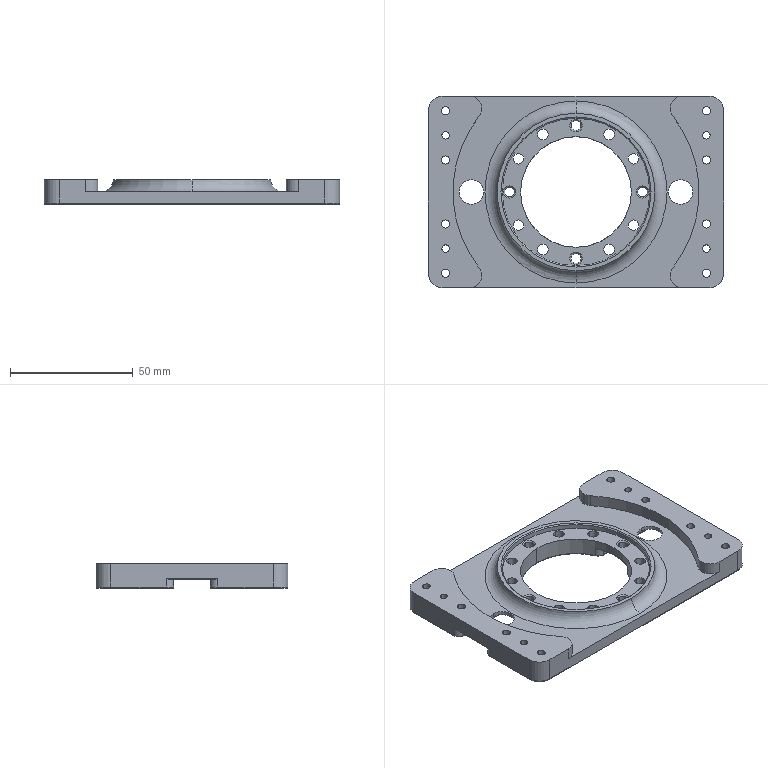NC program | NX | posted with a generic post | part box 120 x 78 x 10 mm
Lines 2931 to 4595 of 5508, first 1393 of 1647 lines:
(ZLEVEL_PROFILE_COPY_1_COPY_COPY_1 , TOOL : D10JING)
N5806 T14 M6
N5808 G54
N5810 G17 G0 G90 X-1.792 Y-15.396 B0. C0. S9500 M3
N5812 G43 Z30. H14
N5814 Z-9.
N5816 G94 G1 Z-10. F1000.
N5818 X-0.866 Y-17.
N5820 G3 X0. Y-17.5 R1.
N5822 X17.5 Y0. R17.5 F1200.
N5824 X0. Y-17.5 R-17.5
N5826 X0.866 Y-17. R1.
N5828 G1 X1.792 Y-15.396
N5830 Z-9.
N5832 G0 Z53.
N5834 X55.67 Y-45.892
N5836 Z-9.
N5838 G1 Z-10. F1000.
N5840 X54.866 Y-44.5
N5842 G3 X54. Y-44. R1.
N5844 G1 X-54. F1200.
N5846 G2 X-65. Y-33. R11.
N5848 G1 Y33.
N5850 G2 X-54. Y44. R11.
N5852 G1 X54.
N5854 G2 X65. Y33. R11.
N5856 G1 Y-33.
N5858 G2 X54. Y-44. R11.
N5860 G3 X53.134 Y-44.5 R1.
N5862 G1 X52.268 Y-46.
N5864 Z-9.
N5866 G0 Z30.
(FLOOR_WALL_COPY , TOOL : D10JING)
N5868 X-66. Y3.974
N5870 Z-2.6
N5872 G1 Z-3.6 F1000.
N5874 X-65.366 Y2.876
N5876 G3 X-64.5 Y2.376 R1.
N5878 G1 X-59.5 F1500.
N5880 G3 X-57. Y2. R8.5
N5882 G1 X-23.238
N5884 G3 X-20.738 Y2.376 R8.5
N5886 G1 X-17.843
N5888 Y-2.376
N5890 X-20.738
N5892 Z-2.6
N5894 G0 Z30.
N5896 Z-2.6
N5898 G1 Z-3.6 F1000.
N5900 G3 X-23.238 Y-2. R8.5
N5902 G1 X-57.
N5904 G3 X-59.5 Y-2.376 R8.5
N5906 G1 X-64.5 F1500.
N5908 G2 X-65.366 Y-1.876 R1.
N5910 G1 X-66. Y-0.778
N5912 Z-2.6
N5914 G0 Z30.
N5916 X-66.286 Y-8.494
N5918 Z-2.6
N5920 G1 Z-3.6 F1000.
N5922 X-65.262 Y-8.324
N5924 G3 X-64.49 Y-7.689 R1.
N5926 G2 X-57. Y-2.5 R8. F1500.
N5928 G1 X-23.238
N5930 G2 X-17.242 Y-5.204 R8.
N5932 G3 X-16.294 Y-5.522 R1.
N5934 G1 Y5.522
N5936 G3 X-17.242 Y5.204 R1. F1000.
N5938 G2 X-23.238 Y2.5 R8. F1500.
N5940 G1 X-57.
N5942 G2 X-64.49 Y7.689 R8.
N5944 G3 X-65.262 Y8.324 R1.
N5946 G1 X-66.286 Y8.494
N5948 Z-2.6
N5950 G0 Z30.
N5952 X16.268 Y2.756
N5954 Z-2.6
N5956 G1 Z-3.6 F1000.
N5958 X16.976 Y2.876
N5960 G3 X17.843 Y2.376 R1.
N5962 G1 X20.738 F1500.
N5964 G3 X23.238 Y2. R8.5
N5966 G1 X57.
N5968 G3 X59.5 Y2.376 R8.5
N5970 G1 X64.5
N5972 Y-2.376
N5974 X59.5
N5976 Z-2.6
N5978 G0 Z30.
N5980 Z-2.6
N5982 G1 Z-3.6 F1000.
N5984 G3 X57. Y-2. R8.5
N5986 G1 X23.238
N5988 G3 X20.738 Y-2.376 R8.5
N5990 G1 X17.843 F1500.
N5992 G2 X16.976 Y-1.876 R1.
N5994 G1 X16.47 Y-0.998
N5996 Z-2.6
N5998 G0 Z30.
N6000 X15.277 Y-5.316
N6002 Z-2.6
N6004 G1 Z-3.6 F1000.
N6006 X16.294 Y-5.522
N6008 G3 X17.242 Y-5.204 R1.
N6010 G2 X23.238 Y-2.5 R8. F1500.
N6012 G1 X57.
N6014 G2 X64.49 Y-7.689 R8.
N6016 G3 X65.262 Y-8.324 R1.
N6018 G1 X66.286 Y-8.494
N6020 Z-2.6
N6022 G0 Z30.
N6024 Y8.494
N6026 Z-2.6
N6028 G1 Z-3.6 F1000.
N6030 X65.262 Y8.324
N6032 G3 X64.49 Y7.689 R1.
N6034 G2 X57. Y2.5 R8. F1500.
N6036 G1 X23.238
N6038 G2 X17.242 Y5.204 R8.
N6040 G3 X16.294 Y5.522 R1.
N6042 G1 X15.277 Y5.316
N6044 Z-2.6
N6046 G0 Z30.
N6048 M5
(HOLE_MILLING , TOOL : D6)
N6050 T12 M6
N6052 G54
N6054 G17 G0 G90 X-42.5 Y0. B0. C0. S9500 M3
N6056 G43 Z30. H12
N6058 Z-3.1
N6060 G94 G3 X-43.5 Y1. R1. F1400.
N6062 X-44.5 Y0. R1.
N6064 X-44.5 Y0. Z-3.45 I2. J0.
N6066 X-44.5 Y0. Z-3.8 I2. J0.
N6068 X-44.5 Y0. Z-4.15 I2. J0.
N6070 X-44.5 Y0. Z-4.5 I2. J0.
N6072 X-44.5 Y0. Z-4.85 I2. J0.
N6074 X-42.055 Y1.95 Z-5.1 R-2.
N6076 X-44.45 Y0.445 R2.
N6078 X-42.055 Y1.95 R-2.
N6080 X-43.252 Y1.197 R1.
N6082 X-42.5 Y0. R1.
N6084 G0 Z30.
N6086 X-23.383 Y13.5
N6088 Z0.5
N6090 G3 X-23.783 Y13.9 R0.4
N6092 X-24.183 Y13.5 R0.4
N6094 X-24.183 Y13.5 Z0.15 I0.8 J0.
N6096 X-24.183 Y13.5 Z-0.2 I0.8 J0.
N6098 X-24.183 Y13.5 Z-0.55 I0.8 J0.
N6100 X-24.183 Y13.5 Z-0.9 I0.8 J0.
N6102 X-24.183 Y13.5 Z-1.25 I0.8 J0.
N6104 X-24.183 Y13.5 Z-1.6 I0.8 J0.
N6106 X-24.183 Y13.5 Z-1.95 I0.8 J0.
N6108 X-24.183 Y13.5 Z-2.3 I0.8 J0.
N6110 X-24.183 Y13.5 Z-2.65 I0.8 J0.
N6112 X-24.183 Y13.5 Z-3. I0.8 J0.
N6114 X-24.183 Y13.5 Z-3.35 I0.8 J0.
N6116 X-24.183 Y13.5 Z-3.7 I0.8 J0.
N6118 X-23.881 Y14.125 Z-4. R-0.8
N6120 X-24.008 Y13.001 R0.8
N6122 X-23.881 Y14.125 R-0.8
N6124 X-23.945 Y13.563 R0.4
N6126 X-23.383 Y13.5 R0.4
N6128 G0 Z30.
N6130 X-13.5 Y23.383
N6132 Z0.5
N6134 G3 X-13.9 Y23.783 R0.4
N6136 X-14.3 Y23.383 R0.4
N6138 X-14.3 Y23.383 Z0.15 I0.8 J0.
N6140 X-14.3 Y23.383 Z-0.2 I0.8 J0.
N6142 X-14.3 Y23.383 Z-0.55 I0.8 J0.
N6144 X-14.3 Y23.383 Z-0.9 I0.8 J0.
N6146 X-14.3 Y23.383 Z-1.25 I0.8 J0.
N6148 X-14.3 Y23.383 Z-1.6 I0.8 J0.
N6150 X-14.3 Y23.383 Z-1.95 I0.8 J0.
N6152 X-14.3 Y23.383 Z-2.3 I0.8 J0.
N6154 X-14.3 Y23.383 Z-2.65 I0.8 J0.
N6156 X-14.3 Y23.383 Z-3. I0.8 J0.
N6158 X-14.3 Y23.383 Z-3.35 I0.8 J0.
N6160 X-14.3 Y23.383 Z-3.7 I0.8 J0.
N6162 X-13.999 Y24.008 Z-4. R-0.8
N6164 X-14.125 Y22.884 R0.8
N6166 X-13.999 Y24.008 R-0.8
N6168 X-14.062 Y23.446 R0.4
N6170 X-13.5 Y23.383 R0.4
N6172 G0 Z30.
N6174 X13.5
N6176 Z0.5
N6178 G3 X13.1 Y23.783 R0.4
N6180 X12.7 Y23.383 R0.4
N6182 X12.7 Y23.383 Z0.15 I0.8 J0.
N6184 X12.7 Y23.383 Z-0.2 I0.8 J0.
N6186 X12.7 Y23.383 Z-0.55 I0.8 J0.
N6188 X12.7 Y23.383 Z-0.9 I0.8 J0.
N6190 X12.7 Y23.383 Z-1.25 I0.8 J0.
N6192 X12.7 Y23.383 Z-1.6 I0.8 J0.
N6194 X12.7 Y23.383 Z-1.95 I0.8 J0.
N6196 X12.7 Y23.383 Z-2.3 I0.8 J0.
N6198 X12.7 Y23.383 Z-2.65 I0.8 J0.
N6200 X12.7 Y23.383 Z-3. I0.8 J0.
N6202 X12.7 Y23.383 Z-3.35 I0.8 J0.
N6204 X12.7 Y23.383 Z-3.7 I0.8 J0.
N6206 X13.001 Y24.008 Z-4. R-0.8
N6208 X12.875 Y22.884 R0.8
N6210 X13.001 Y24.008 R-0.8
N6212 X12.938 Y23.446 R0.4
N6214 X13.5 Y23.383 R0.4
N6216 G0 Z30.
N6218 X23.383 Y13.5
N6220 Z0.5
N6222 G3 X22.983 Y13.9 R0.4
N6224 X22.583 Y13.5 R0.4
N6226 X22.583 Y13.5 Z0.15 I0.8 J0.
N6228 X22.583 Y13.5 Z-0.2 I0.8 J0.
N6230 X22.583 Y13.5 Z-0.55 I0.8 J0.
N6232 X22.583 Y13.5 Z-0.9 I0.8 J0.
N6234 X22.583 Y13.5 Z-1.25 I0.8 J0.
N6236 X22.583 Y13.5 Z-1.6 I0.8 J0.
N6238 X22.583 Y13.5 Z-1.95 I0.8 J0.
N6240 X22.583 Y13.5 Z-2.3 I0.8 J0.
N6242 X22.583 Y13.5 Z-2.65 I0.8 J0.
N6244 X22.583 Y13.5 Z-3. I0.8 J0.
N6246 X22.583 Y13.5 Z-3.35 I0.8 J0.
N6248 X22.583 Y13.5 Z-3.7 I0.8 J0.
N6250 X22.884 Y14.125 Z-4. R-0.8
N6252 X22.757 Y13.001 R0.8
N6254 X22.884 Y14.125 R-0.8
N6256 X22.821 Y13.563 R0.4
N6258 X23.383 Y13.5 R0.4
N6260 G0 Z30.
N6262 X42.5 Y0.
N6264 Z-3.1
N6266 G3 X41.5 Y1. R1.
N6268 X40.5 Y0. R1.
N6270 X40.5 Y0. Z-3.45 I2. J0.
N6272 X40.5 Y0. Z-3.8 I2. J0.
N6274 X40.5 Y0. Z-4.15 I2. J0.
N6276 X40.5 Y0. Z-4.5 I2. J0.
N6278 X40.5 Y0. Z-4.85 I2. J0.
N6280 X42.945 Y1.95 Z-5.1 R-2.
N6282 X40.55 Y0.445 R2.
N6284 X42.945 Y1.95 R-2.
N6286 X41.748 Y1.197 R1.
N6288 X42.5 Y0. R1.
N6290 G0 Z30.
N6292 X23.383 Y-13.5
N6294 Z0.5
N6296 G3 X22.983 Y-13.1 R0.4
N6298 X22.583 Y-13.5 R0.4
N6300 X22.583 Y-13.5 Z0.15 I0.8 J0.
N6302 X22.583 Y-13.5 Z-0.2 I0.8 J0.
N6304 X22.583 Y-13.5 Z-0.55 I0.8 J0.
N6306 X22.583 Y-13.5 Z-0.9 I0.8 J0.
N6308 X22.583 Y-13.5 Z-1.25 I0.8 J0.
N6310 X22.583 Y-13.5 Z-1.6 I0.8 J0.
N6312 X22.583 Y-13.5 Z-1.95 I0.8 J0.
N6314 X22.583 Y-13.5 Z-2.3 I0.8 J0.
N6316 X22.583 Y-13.5 Z-2.65 I0.8 J0.
N6318 X22.583 Y-13.5 Z-3. I0.8 J0.
N6320 X22.583 Y-13.5 Z-3.35 I0.8 J0.
N6322 X22.583 Y-13.5 Z-3.7 I0.8 J0.
N6324 X22.884 Y-12.875 Z-4. R-0.8
N6326 X22.757 Y-13.999 R0.8
N6328 X22.884 Y-12.875 R-0.8
N6330 X22.821 Y-13.437 R0.4
N6332 X23.383 Y-13.5 R0.4
N6334 G0 Z30.
N6336 X13.5 Y-23.383
N6338 Z0.5
N6340 G3 X13.1 Y-22.983 R0.4
N6342 X12.7 Y-23.383 R0.4
N6344 X12.7 Y-23.383 Z0.15 I0.8 J0.
N6346 X12.7 Y-23.383 Z-0.2 I0.8 J0.
N6348 X12.7 Y-23.383 Z-0.55 I0.8 J0.
N6350 X12.7 Y-23.383 Z-0.9 I0.8 J0.
N6352 X12.7 Y-23.383 Z-1.25 I0.8 J0.
N6354 X12.7 Y-23.383 Z-1.6 I0.8 J0.
N6356 X12.7 Y-23.383 Z-1.95 I0.8 J0.
N6358 X12.7 Y-23.383 Z-2.3 I0.8 J0.
N6360 X12.7 Y-23.383 Z-2.65 I0.8 J0.
N6362 X12.7 Y-23.383 Z-3. I0.8 J0.
N6364 X12.7 Y-23.383 Z-3.35 I0.8 J0.
N6366 X12.7 Y-23.383 Z-3.7 I0.8 J0.
N6368 X13.001 Y-22.757 Z-4. R-0.8
N6370 X12.875 Y-23.881 R0.8
N6372 X13.001 Y-22.757 R-0.8
N6374 X12.938 Y-23.319 R0.4
N6376 X13.5 Y-23.383 R0.4
N6378 G0 Z30.
N6380 X-13.5
N6382 Z0.5
N6384 G3 X-13.9 Y-22.983 R0.4
N6386 X-14.3 Y-23.383 R0.4
N6388 X-14.3 Y-23.383 Z0.15 I0.8 J0.
N6390 X-14.3 Y-23.383 Z-0.2 I0.8 J0.
N6392 X-14.3 Y-23.383 Z-0.55 I0.8 J0.
N6394 X-14.3 Y-23.383 Z-0.9 I0.8 J0.
N6396 X-14.3 Y-23.383 Z-1.25 I0.8 J0.
N6398 X-14.3 Y-23.383 Z-1.6 I0.8 J0.
N6400 X-14.3 Y-23.383 Z-1.95 I0.8 J0.
N6402 X-14.3 Y-23.383 Z-2.3 I0.8 J0.
N6404 X-14.3 Y-23.383 Z-2.65 I0.8 J0.
N6406 X-14.3 Y-23.383 Z-3. I0.8 J0.
N6408 X-14.3 Y-23.383 Z-3.35 I0.8 J0.
N6410 X-14.3 Y-23.383 Z-3.7 I0.8 J0.
N6412 X-13.999 Y-22.757 Z-4. R-0.8
N6414 X-14.125 Y-23.881 R0.8
N6416 X-13.999 Y-22.757 R-0.8
N6418 X-14.062 Y-23.319 R0.4
N6420 X-13.5 Y-23.383 R0.4
N6422 G0 Z30.
N6424 X-23.383 Y-13.5
N6426 Z0.5
N6428 G3 X-23.783 Y-13.1 R0.4
N6430 X-24.183 Y-13.5 R0.4
N6432 X-24.183 Y-13.5 Z0.15 I0.8 J0.
N6434 X-24.183 Y-13.5 Z-0.2 I0.8 J0.
N6436 X-24.183 Y-13.5 Z-0.55 I0.8 J0.
N6438 X-24.183 Y-13.5 Z-0.9 I0.8 J0.
N6440 X-24.183 Y-13.5 Z-1.25 I0.8 J0.
N6442 X-24.183 Y-13.5 Z-1.6 I0.8 J0.
N6444 X-24.183 Y-13.5 Z-1.95 I0.8 J0.
N6446 X-24.183 Y-13.5 Z-2.3 I0.8 J0.
N6448 X-24.183 Y-13.5 Z-2.65 I0.8 J0.
N6450 X-24.183 Y-13.5 Z-3. I0.8 J0.
N6452 X-24.183 Y-13.5 Z-3.35 I0.8 J0.
N6454 X-24.183 Y-13.5 Z-3.7 I0.8 J0.
N6456 X-23.881 Y-12.875 Z-4. R-0.8
N6458 X-24.008 Y-13.999 R0.8
N6460 X-23.881 Y-12.875 R-0.8
N6462 X-23.945 Y-13.437 R0.4
N6464 X-23.383 Y-13.5 R0.4
N6466 G0 Z30.
(ZLEVEL_PROFILE , TOOL : D6)
N6468 X-27.332 Y-29.8
N6470 Z-0.4
N6472 G1 X-26.813 Y-30.7 F2000.
N6474 G3 X-26.293 Y-31. R0.6
N6476 G1 X-20.199
N6478 G2 X-24.906 Y-27.363 R37.
N6480 G3 X-25.492 Y-27.235 R0.6
N6482 G1 X-26.466 Y-27.546
N6484 G0 X-27.332 Y-29.8 Z-0.8
N6486 G1 X-26.813 Y-30.7
N6488 G3 X-26.293 Y-31. R0.6
N6490 G1 X-20.199
N6492 G2 X-24.906 Y-27.363 R37.
N6494 G3 X-25.492 Y-27.235 R0.6
N6496 G1 X-26.466 Y-27.546
N6498 G0 X-27.332 Y-29.8 Z-1.2
N6500 G1 X-26.813 Y-30.7
N6502 G3 X-26.293 Y-31. R0.6
N6504 G1 X-20.199
N6506 G2 X-24.906 Y-27.363 R37.
N6508 G3 X-25.492 Y-27.235 R0.6
N6510 G1 X-26.466 Y-27.546
N6512 G0 X-27.332 Y-29.8 Z-1.6
N6514 G1 X-26.813 Y-30.7
N6516 G3 X-26.293 Y-31. R0.6
N6518 G1 X-20.199
N6520 G2 X-24.906 Y-27.363 R37.
N6522 G3 X-25.492 Y-27.235 R0.6
N6524 G1 X-26.466 Y-27.546
N6526 G0 Z30.
N6528 X-33.553 Y-18.26
N6530 Z-0.4
N6532 G1 X-32.996 Y-17.401
N6534 G3 X-32.965 Y-16.802 R0.6
N6536 G2 X-33.597 Y-15.5 R37.
N6538 G1 X-35.07
N6540 G3 X-35.589 Y-15.8 R0.6
N6542 G1 X-36.109 Y-16.7
N6544 G0 X-33.553 Y-18.26 Z-0.8
N6546 G1 X-32.996 Y-17.401
N6548 G3 X-32.965 Y-16.802 R0.6
N6550 G2 X-33.597 Y-15.5 R37.
N6552 G1 X-35.07
N6554 G3 X-35.589 Y-15.8 R0.6
N6556 G1 X-36.109 Y-16.7
N6558 G0 X-33.553 Y-18.26 Z-1.2
N6560 G1 X-32.996 Y-17.401
N6562 G3 X-32.965 Y-16.802 R0.6
N6564 G2 X-33.597 Y-15.5 R37.
N6566 G1 X-35.07
N6568 G3 X-35.589 Y-15.8 R0.6
N6570 G1 X-36.109 Y-16.7
N6572 G0 X-33.553 Y-18.26 Z-1.6
N6574 G1 X-32.996 Y-17.401
N6576 G3 X-32.965 Y-16.802 R0.6
N6578 G2 X-33.597 Y-15.5 R37.
N6580 G1 X-35.07
N6582 G3 X-35.589 Y-15.8 R0.6
N6584 G1 X-36.109 Y-16.7
N6586 G0 Z30.
N6588 X-41.744
N6590 Z-0.4
N6592 G1 X-42.264 Y-15.8
N6594 G3 X-42.784 Y-15.5 R0.6
N6596 G1 X-45.
N6598 Y-17.716
N6600 G3 X-44.7 Y-18.236 R0.6
N6602 G1 X-43.8 Y-18.756
N6604 G0 X-41.744 Y-16.7 Z-0.8
N6606 G1 X-42.264 Y-15.8
N6608 G3 X-42.784 Y-15.5 R0.6
N6610 G1 X-45.
N6612 Y-17.716
N6614 G3 X-44.7 Y-18.236 R0.6
N6616 G1 X-43.8 Y-18.756
N6618 G0 X-41.744 Y-16.7 Z-1.2
N6620 G1 X-42.264 Y-15.8
N6622 G3 X-42.784 Y-15.5 R0.6
N6624 G1 X-45.
N6626 Y-17.716
N6628 G3 X-44.7 Y-18.236 R0.6
N6630 G1 X-43.8 Y-18.756
N6632 G0 X-41.744 Y-16.7 Z-1.6
N6634 G1 X-42.264 Y-15.8
N6636 G3 X-42.784 Y-15.5 R0.6
N6638 G1 X-45.
N6640 Y-17.716
N6642 G3 X-44.7 Y-18.236 R0.6
N6644 G1 X-43.8 Y-18.756
N6646 G0 Z30.
N6648 Y-27.744
N6650 Z-0.4
N6652 G1 X-44.7 Y-28.264
N6654 G3 X-45. Y-28.783 R0.6
N6656 G1 Y-31.
N6658 X-42.783
N6660 G3 X-42.264 Y-30.7 R0.6
N6662 G1 X-41.744 Y-29.8
N6664 G0 X-43.8 Y-27.744 Z-0.8
N6666 G1 X-44.7 Y-28.264
N6668 G3 X-45. Y-28.783 R0.6
N6670 G1 Y-31.
N6672 X-42.783
N6674 G3 X-42.264 Y-30.7 R0.6
N6676 G1 X-41.744 Y-29.8
N6678 G0 X-43.8 Y-27.744 Z-1.2
N6680 G1 X-44.7 Y-28.263
N6682 G3 X-45. Y-28.783 R0.6
N6684 G1 Y-31.
N6686 X-42.783
N6688 G3 X-42.263 Y-30.7 R0.6
N6690 G1 X-41.744 Y-29.8
N6692 G0 X-43.8 Y-27.744 Z-1.6
N6694 G1 X-44.7 Y-28.263
N6696 G3 X-45. Y-28.783 R0.6
N6698 G1 Y-31.
N6700 X-42.783
N6702 G3 X-42.263 Y-30.7 R0.6
N6704 G1 X-41.744 Y-29.8
N6706 G0 Z30.
N6708 X-36.109 Y16.7
N6710 Z-0.4
N6712 G1 X-35.59 Y15.8
N6714 G3 X-35.07 Y15.5 R0.6
N6716 G1 X-33.597
N6718 G2 X-32.965 Y16.802 R37.
N6720 G3 X-32.996 Y17.402 R0.6
N6722 G1 X-33.553 Y18.26
N6724 G0 X-36.109 Y16.7 Z-0.8
N6726 G1 X-35.59 Y15.8
N6728 G3 X-35.07 Y15.5 R0.6
N6730 G1 X-33.597
N6732 G2 X-32.965 Y16.803 R37.
N6734 G3 X-32.996 Y17.402 R0.6
N6736 G1 X-33.553 Y18.26
N6738 G0 X-36.109 Y16.7 Z-1.2
N6740 G1 X-35.59 Y15.8
N6742 G3 X-35.07 Y15.5 R0.6
N6744 G1 X-33.597
N6746 G2 X-32.965 Y16.803 R37.
N6748 G3 X-32.996 Y17.402 R0.6
N6750 G1 X-33.553 Y18.26
N6752 G0 X-36.11 Y16.7 Z-1.6
N6754 G1 X-35.59 Y15.8
N6756 G3 X-35.07 Y15.5 R0.6
N6758 G1 X-33.597
N6760 G2 X-32.965 Y16.803 R37.
N6762 G3 X-32.996 Y17.402 R0.6
N6764 G1 X-33.553 Y18.26
N6766 G0 Z30.
N6768 X-26.466 Y27.546
N6770 Z-0.4
N6772 G1 X-25.492 Y27.235
N6774 G3 X-24.906 Y27.363 R0.6
N6776 G2 X-20.197 Y31.001 R37.
N6778 G1 X-26.293 Y31.
N6780 G3 X-26.813 Y30.7 R0.6
N6782 G1 X-27.332 Y29.8
N6784 G0 X-26.466 Y27.546 Z-0.8
N6786 G1 X-25.492 Y27.235
N6788 G3 X-24.906 Y27.363 R0.6
N6790 G2 X-20.198 Y31.001 R37.
N6792 G1 X-26.293 Y31.
N6794 G3 X-26.813 Y30.7 R0.6
N6796 G1 X-27.332 Y29.8
N6798 G0 X-26.466 Y27.546 Z-1.2
N6800 G1 X-25.492 Y27.235
N6802 G3 X-24.906 Y27.363 R0.6
N6804 G2 X-20.199 Y31. R37.
N6806 G1 X-26.293
N6808 G3 X-26.813 Y30.7 R0.6
N6810 G1 X-27.332 Y29.8
N6812 G0 X-26.466 Y27.546 Z-1.6
N6814 G1 X-25.492 Y27.235
N6816 G3 X-24.906 Y27.363 R0.6
N6818 G2 X-20.2 Y31. R37.
N6820 G1 X-26.293
N6822 G3 X-26.813 Y30.7 R0.6
N6824 G1 X-27.332 Y29.8
N6826 G0 Z30.
N6828 X-41.744
N6830 Z-0.4
N6832 G1 X-42.264 Y30.7
N6834 G3 X-42.784 Y31. R0.6
N6836 G1 X-45.
N6838 Y28.784
N6840 G3 X-44.7 Y28.264 R0.6
N6842 G1 X-43.8 Y27.744
N6844 G0 X-41.744 Y29.8 Z-0.8
N6846 G1 X-42.264 Y30.7
N6848 G3 X-42.784 Y31. R0.6
N6850 G1 X-45.
N6852 Y28.784
N6854 G3 X-44.7 Y28.264 R0.6
N6856 G1 X-43.8 Y27.744
N6858 G0 X-41.744 Y29.8 Z-1.2
N6860 G1 X-42.264 Y30.7
N6862 G3 X-42.784 Y31. R0.6
N6864 G1 X-45.
N6866 Y28.784
N6868 G3 X-44.7 Y28.264 R0.6
N6870 G1 X-43.8 Y27.744
N6872 G0 X-41.744 Y29.8 Z-1.6
N6874 G1 X-42.264 Y30.7
N6876 G3 X-42.784 Y31. R0.6
N6878 G1 X-45.
N6880 Y28.784
N6882 G3 X-44.7 Y28.264 R0.6
N6884 G1 X-43.8 Y27.744
N6886 G0 Z30.
N6888 Y18.756
N6890 Z-0.4
N6892 G1 X-44.7 Y18.236
N6894 G3 X-45. Y17.717 R0.6
N6896 G1 Y15.5
N6898 X-42.783
N6900 G3 X-42.264 Y15.8 R0.6
N6902 G1 X-41.744 Y16.7
N6904 G0 X-43.8 Y18.756 Z-0.8
N6906 G1 X-44.7 Y18.237
N6908 G3 X-45. Y17.717 R0.6
N6910 G1 Y15.5
N6912 X-42.783
N6914 G3 X-42.263 Y15.8 R0.6
N6916 G1 X-41.744 Y16.7
N6918 G0 X-43.8 Y18.757 Z-1.2
N6920 G1 X-44.7 Y18.237
N6922 G3 X-45. Y17.717 R0.6
N6924 G1 Y15.5
N6926 X-42.783
N6928 G3 X-42.263 Y15.8 R0.6
N6930 G1 X-41.743 Y16.7
N6932 G0 X-43.8 Y18.757 Z-1.6
N6934 G1 X-44.7 Y18.237
N6936 G3 X-45. Y17.718 R0.6
N6938 G1 Y15.5
N6940 X-42.782
N6942 G3 X-42.263 Y15.8 R0.6
N6944 G1 X-41.743 Y16.7
N6946 G0 Z30.
N6948 X41.744
N6950 Z-0.4
N6952 G1 X42.264 Y15.8
N6954 G3 X42.784 Y15.5 R0.6
N6956 G1 X45.
N6958 Y17.716
N6960 G3 X44.7 Y18.236 R0.6
N6962 G1 X43.8 Y18.756
N6964 G0 X41.744 Y16.7 Z-0.8
N6966 G1 X42.264 Y15.8
N6968 G3 X42.784 Y15.5 R0.6
N6970 G1 X45.
N6972 Y17.716
N6974 G3 X44.7 Y18.236 R0.6
N6976 G1 X43.8 Y18.756
N6978 G0 X41.744 Y16.7 Z-1.2
N6980 G1 X42.264 Y15.8
N6982 G3 X42.784 Y15.5 R0.6
N6984 G1 X45.
N6986 Y17.716
N6988 G3 X44.7 Y18.236 R0.6
N6990 G1 X43.8 Y18.756
N6992 G0 X41.744 Y16.7 Z-1.6
N6994 G1 X42.264 Y15.8
N6996 G3 X42.784 Y15.5 R0.6
N6998 G1 X45.
N7000 Y17.716
N7002 G3 X44.7 Y18.236 R0.6
N7004 G1 X43.8 Y18.756
N7006 G0 Z30.
N7008 Y27.744
N7010 Z-0.4
N7012 G1 X44.7 Y28.264
N7014 G3 X45. Y28.784 R0.6
N7016 G1 Y31.
N7018 X42.784
N7020 G3 X42.264 Y30.7 R0.6
N7022 G1 X41.744 Y29.8
N7024 G0 X43.8 Y27.744 Z-0.8
N7026 G1 X44.7 Y28.264
N7028 G3 X45. Y28.784 R0.6
N7030 G1 Y31.
N7032 X42.784
N7034 G3 X42.264 Y30.7 R0.6
N7036 G1 X41.744 Y29.8
N7038 G0 X43.8 Y27.744 Z-1.2
N7040 G1 X44.7 Y28.264
N7042 G3 X45. Y28.784 R0.6
N7044 G1 Y31.
N7046 X42.784
N7048 G3 X42.264 Y30.7 R0.6
N7050 G1 X41.744 Y29.8
N7052 G0 X43.8 Y27.744 Z-1.6
N7054 G1 X44.7 Y28.264
N7056 G3 X45. Y28.784 R0.6
N7058 G1 Y31.
N7060 X42.784
N7062 G3 X42.264 Y30.7 R0.6
N7064 G1 X41.744 Y29.8
N7066 G0 Z30.
N7068 X27.332
N7070 Z-0.4
N7072 G1 X26.813 Y30.7
N7074 G3 X26.293 Y31. R0.6
N7076 G1 X20.197 Y31.001
N7078 G2 X24.906 Y27.363 R37.
N7080 G3 X25.492 Y27.235 R0.6
N7082 G1 X26.466 Y27.546
N7084 G0 X27.332 Y29.8 Z-0.8
N7086 G1 X26.813 Y30.7
N7088 G3 X26.293 Y31. R0.6
N7090 G1 X20.198 Y31.001
N7092 G2 X24.906 Y27.363 R37.
N7094 G3 X25.492 Y27.235 R0.6
N7096 G1 X26.466 Y27.546
N7098 G0 X27.332 Y29.8 Z-1.2
N7100 G1 X26.813 Y30.7
N7102 G3 X26.293 Y31. R0.6
N7104 G1 X20.199
N7106 G2 X24.906 Y27.363 R37.
N7108 G3 X25.492 Y27.235 R0.6
N7110 G1 X26.466 Y27.546
N7112 G0 X27.332 Y29.8 Z-1.6
N7114 G1 X26.813 Y30.7
N7116 G3 X26.293 Y31. R0.6
N7118 G1 X20.2
N7120 G2 X24.906 Y27.363 R37.
N7122 G3 X25.492 Y27.235 R0.6
N7124 G1 X26.466 Y27.546
N7126 G0 Z30.
N7128 X33.553 Y18.26
N7130 Z-0.4
N7132 G1 X32.996 Y17.402
N7134 G3 X32.965 Y16.802 R0.6
N7136 G2 X33.597 Y15.5 R37.
N7138 G1 X35.07
N7140 G3 X35.59 Y15.8 R0.6
N7142 G1 X36.109 Y16.7
N7144 G0 X33.553 Y18.26 Z-0.8
N7146 G1 X32.996 Y17.402
N7148 G3 X32.965 Y16.803 R0.6
N7150 G2 X33.597 Y15.5 R37.
N7152 G1 X35.07
N7154 G3 X35.59 Y15.8 R0.6
N7156 G1 X36.109 Y16.7
N7158 G0 X33.553 Y18.26 Z-1.2
N7160 G1 X32.996 Y17.402
N7162 G3 X32.965 Y16.803 R0.6
N7164 G2 X33.597 Y15.5 R37.
N7166 G1 X35.07
N7168 G3 X35.59 Y15.8 R0.6
N7170 G1 X36.109 Y16.7
N7172 G0 X33.553 Y18.26 Z-1.6
N7174 G1 X32.996 Y17.402
N7176 G3 X32.965 Y16.803 R0.6
N7178 G2 X33.597 Y15.5 R37.
N7180 G1 X35.07
N7182 G3 X35.59 Y15.8 R0.6
N7184 G1 X36.11 Y16.7
N7186 G0 Z30.
N7188 X41.744 Y-29.8
N7190 Z-0.4
N7192 G1 X42.264 Y-30.7
N7194 G3 X42.784 Y-31. R0.6
N7196 G1 X45.
N7198 Y-28.784
N7200 G3 X44.7 Y-28.264 R0.6
N7202 G1 X43.8 Y-27.744
N7204 G0 X41.744 Y-29.8 Z-0.8
N7206 G1 X42.264 Y-30.7
N7208 G3 X42.784 Y-31. R0.6
N7210 G1 X45.
N7212 Y-28.784
N7214 G3 X44.7 Y-28.264 R0.6
N7216 G1 X43.8 Y-27.744
N7218 G0 X41.744 Y-29.8 Z-1.2
N7220 G1 X42.264 Y-30.7
N7222 G3 X42.784 Y-31. R0.6
N7224 G1 X45.
N7226 Y-28.784
N7228 G3 X44.7 Y-28.264 R0.6
N7230 G1 X43.8 Y-27.744
N7232 G0 X41.744 Y-29.8 Z-1.6
N7234 G1 X42.264 Y-30.7
N7236 G3 X42.784 Y-31. R0.6
N7238 G1 X45.
N7240 Y-28.784
N7242 G3 X44.7 Y-28.264 R0.6
N7244 G1 X43.8 Y-27.744
N7246 G0 Z30.
N7248 Y-18.756
N7250 Z-0.4
N7252 G1 X44.7 Y-18.236
N7254 G3 X45. Y-17.717 R0.6
N7256 G1 Y-15.5
N7258 X42.783
N7260 G3 X42.264 Y-15.8 R0.6
N7262 G1 X41.744 Y-16.7
N7264 G0 X43.8 Y-18.756 Z-0.8
N7266 G1 X44.7 Y-18.236
N7268 G3 X45. Y-17.717 R0.6
N7270 G1 Y-15.5
N7272 X42.783
N7274 G3 X42.264 Y-15.8 R0.6
N7276 G1 X41.744 Y-16.7
N7278 G0 X43.8 Y-18.756 Z-1.2
N7280 G1 X44.7 Y-18.236
N7282 G3 X45. Y-17.717 R0.6
N7284 G1 Y-15.5
N7286 X42.783
N7288 G3 X42.264 Y-15.8 R0.6
N7290 G1 X41.744 Y-16.7
N7292 G0 X43.8 Y-18.756 Z-1.6
N7294 G1 X44.7 Y-18.236
N7296 G3 X45. Y-17.717 R0.6
N7298 G1 Y-15.5
N7300 X42.783
N7302 G3 X42.264 Y-15.8 R0.6
N7304 G1 X41.744 Y-16.7
N7306 G0 Z30.
N7308 X36.109
N7310 Z-0.4
N7312 G1 X35.589 Y-15.8
N7314 G3 X35.07 Y-15.5 R0.6
N7316 G1 X33.597
N7318 G2 X32.965 Y-16.802 R37.
N7320 G3 X32.996 Y-17.401 R0.6
N7322 G1 X33.553 Y-18.26
N7324 G0 X36.109 Y-16.7 Z-0.8
N7326 G1 X35.589 Y-15.8
N7328 G3 X35.07 Y-15.5 R0.6
N7330 G1 X33.597
N7332 G2 X32.965 Y-16.802 R37.
N7334 G3 X32.996 Y-17.401 R0.6
N7336 G1 X33.553 Y-18.26
N7338 G0 X36.109 Y-16.7 Z-1.2
N7340 G1 X35.589 Y-15.8
N7342 G3 X35.07 Y-15.5 R0.6
N7344 G1 X33.597
N7346 G2 X32.965 Y-16.802 R37.
N7348 G3 X32.996 Y-17.401 R0.6
N7350 G1 X33.553 Y-18.26
N7352 G0 X36.109 Y-16.7 Z-1.6
N7354 G1 X35.589 Y-15.8
N7356 G3 X35.07 Y-15.5 R0.6
N7358 G1 X33.597
N7360 G2 X32.965 Y-16.802 R37.
N7362 G3 X32.996 Y-17.401 R0.6
N7364 G1 X33.553 Y-18.26
N7366 G0 Z30.
N7368 X26.467 Y-27.546
N7370 Z-0.4
N7372 G1 X25.492 Y-27.235
N7374 G3 X24.906 Y-27.363 R0.6
N7376 G2 X20.561 Y-30.761 R37.
N7378 G1 X20.221 Y-30.986
N7380 X20.199 Y-31.
N7382 X26.293
N7384 G3 X26.813 Y-30.7 R0.6
N7386 G1 X27.333 Y-29.8
N7388 G0 X26.467 Y-27.546 Z-0.8
N7390 G1 X25.492 Y-27.235
N7392 G3 X24.906 Y-27.363 R0.6
N7394 G2 X20.561 Y-30.761 R37.
N7396 G1 X20.221 Y-30.986
N7398 X20.199 Y-31.
N7400 X26.293
N7402 G3 X26.813 Y-30.7 R0.6
N7404 G1 X27.333 Y-29.8
N7406 G0 X26.467 Y-27.545 Z-1.2
N7408 G1 X25.492 Y-27.235
N7410 G3 X24.906 Y-27.362 R0.6
N7412 G2 X20.221 Y-30.985 R37.
N7414 G1 X20.217 Y-30.988
N7416 X20.199 Y-31.
N7418 X26.294
N7420 G3 X26.813 Y-30.7 R0.6
N7422 G1 X27.333 Y-29.8
N7424 G0 X26.467 Y-27.545 Z-1.6
N7426 G1 X25.492 Y-27.234
N7428 G3 X24.906 Y-27.362 R0.6
N7430 G2 X20.222 Y-30.985 R37.
N7432 G1 X20.217 Y-30.988
N7434 X20.199 Y-31.
N7436 X26.294
N7438 G3 X26.813 Y-30.7 R0.6
N7440 G1 X27.333 Y-29.8
N7442 G0 Z30.
(FLOOR_WALL_COPY_COPY , TOOL : D6)
N7444 X-44.18 Y30.399
N7446 Z-0.6
N7448 G1 Z-1.6 F1000.
N7450 G3 X-44.7 Y30.699 R0.6
N7452 G1 X-21.186 F1500.
N7454 G3 X-24.959 Y27.719 R37.3
N7456 G1 X-44.7
N7458 Y24.739
N7460 X-27.915
N7462 G3 X-30.295 Y21.76 R37.3
N7464 G1 X-44.7
N7466 Y18.78
N7468 X-32.227
N7470 G3 X-33.788 Y15.8 R37.3
N7472 G1 X-44.7
N7474 Y16.32
N7476 G3 X-45. Y15.8 R0.6 F1000.
N7478 G1 Y15.5 F1500.
N7480 X-33.597
N7482 G2 X-20.199 Y31. R37.
N7484 G1 X-45.
N7486 Y15.8
N7488 G3 X-44.85 Y15.54 R0.3
N7490 G1 X-43.5 Y17.
N7492 Z-0.6
N7494 G0 Z30.
N7496 X-44.18 Y-16.101
N7498 Z-0.6
N7500 G1 Z-1.6 F1000.
N7502 G3 X-44.7 Y-15.801 R0.6
N7504 G1 X-33.788 F1500.
N7506 G3 X-32.227 Y-18.781 R37.3
N7508 G1 X-44.7
N7510 Y-21.761
N7512 X-30.295
N7514 G3 X-27.914 Y-24.74 R37.3
N7516 G1 X-44.7
N7518 Y-27.72
N7520 X-24.958
N7522 G3 X-21.185 Y-30.7 R37.3
N7524 G1 X-44.7
N7526 Y-30.18
N7528 G3 X-45. Y-30.7 R0.6 F1000.
N7530 G1 Y-31. F1500.
N7532 X-20.199
N7534 G2 X-33.597 Y-15.5 R37.
N7536 G1 X-45.
N7538 Y-30.7
N7540 G3 X-44.85 Y-30.96 R0.3
N7542 G1 X-43.5 Y-29.5
N7544 Z-0.6
N7546 G0 Z30.
N7548 X34.307 Y-16.101
N7550 Z-0.6
N7552 G1 Z-1.6 F1000.
N7554 G3 X33.788 Y-15.801 R0.6
N7556 G1 X44.7 F1500.
N7558 Y-18.781
N7560 X32.227
N7562 G2 X30.295 Y-21.761 R37.3
N7564 G1 X44.7
N7566 Y-24.74
N7568 X27.914
N7570 G2 X24.958 Y-27.72 R37.3
N7572 G1 X44.7
N7574 Y-30.7
N7576 X21.185
N7578 X21.613 Y-30.405
N7580 G3 X21.015 Y-30.453 R0.6 F1000.
N7582 G2 X20.199 Y-31. R37. F1500.
N7584 G1 X45.
N7586 Y-15.5
N7588 X33.597
N7590 G2 X21.015 Y-30.453 R37.
N7592 G3 X20.757 Y-30.995 R0.6
N7594 G1 X24.739 Y-29.5
N7596 Z-0.6
N7598 G0 Z30.
N7600 X21.706 Y30.399
N7602 Z-0.6
N7604 G1 Z-1.6 F1000.
N7606 G3 X21.186 Y30.699 R0.6
N7608 G1 X44.7 F1500.
N7610 Y27.719
N7612 X24.959
N7614 G2 X27.915 Y24.739 R37.3
N7616 G1 X44.7
N7618 Y21.76
N7620 X30.295
N7622 G2 X32.227 Y18.78 R37.3
N7624 G1 X44.7
N7626 Y15.8
N7628 X33.788
N7630 X33.568 Y16.271
N7632 G3 X33.517 Y15.673 R0.6 F1000.
N7634 G1 X33.597 Y15.5 F1500.
N7636 X45.
N7638 Y31.
N7640 X20.199
N7642 G2 X33.517 Y15.673 R37.
N7644 G3 X33.762 Y15.501 R0.3
N7646 G1 X34.543 Y17.
N7648 Z-0.6
N7650 G0 Z30.
N7652 M5
(HOLE_MILLING_1 , TOOL : D3)
N7654 T17 M6
N7656 G54
N7658 G17 G0 G90 X-53. Y23. B0. C0. S9500 M3
N7660 G43 Z30. H17
N7662 Z0.5
N7664 G94 G3 X-53.2 Y23.2 R0.2 F1250.
N7666 X-53.4 Y23. R0.2
N7668 X-53.4 Y23. Z0.25 I0.4 J0.
N7670 X-53.4 Y23. Z0. I0.4 J0.
N7672 X-53.4 Y23. Z-0.25 I0.4 J0.
N7674 X-53.4 Y23. Z-0.5 I0.4 J0.
N7676 X-53.4 Y23. Z-0.75 I0.4 J0.
N7678 X-53.4 Y23. Z-1. I0.4 J0.
N7680 X-53.4 Y23. Z-1.25 I0.4 J0.
N7682 X-53.4 Y23. Z-1.5 I0.4 J0.
N7684 X-53.4 Y23. Z-1.75 I0.4 J0.
N7686 X-53.4 Y23. Z-2. I0.4 J0.
N7688 X-53.4 Y23. Z-2.25 I0.4 J0.
N7690 X-53.4 Y23. Z-2.5 I0.4 J0.
N7692 X-53.4 Y23. Z-2.75 I0.4 J0.
N7694 X-53.4 Y23. Z-3. I0.4 J0.
N7696 X-53.4 Y23. Z-3.25 I0.4 J0.
N7698 X-53.4 Y23. Z-3.5 I0.4 J0.
N7700 X-53.4 Y23. Z-3.75 I0.4 J0.
N7702 X-53.4 Y23. Z-4. I0.4 J0.
N7704 X-53. Y22.6 R0.4
N7706 X-53.4 Y23. R-0.4
N7708 X-53.2 Y22.8 R0.2
N7710 X-53. Y23. R0.2
N7712 G0 Z30.
N7714 Y-23.
N7716 Z0.5
N7718 G3 X-53.2 Y-22.8 R0.2
N7720 X-53.4 Y-23. R0.2
N7722 X-53.4 Y-23. Z0.25 I0.4 J0.
N7724 X-53.4 Y-23. Z0. I0.4 J0.
N7726 X-53.4 Y-23. Z-0.25 I0.4 J0.
N7728 X-53.4 Y-23. Z-0.5 I0.4 J0.
N7730 X-53.4 Y-23. Z-0.75 I0.4 J0.
N7732 X-53.4 Y-23. Z-1. I0.4 J0.
N7734 X-53.4 Y-23. Z-1.25 I0.4 J0.
N7736 X-53.4 Y-23. Z-1.5 I0.4 J0.
N7738 X-53.4 Y-23. Z-1.75 I0.4 J0.
N7740 X-53.4 Y-23. Z-2. I0.4 J0.
N7742 X-53.4 Y-23. Z-2.25 I0.4 J0.
N7744 X-53.4 Y-23. Z-2.5 I0.4 J0.
N7746 X-53.4 Y-23. Z-2.75 I0.4 J0.
N7748 X-53.4 Y-23. Z-3. I0.4 J0.
N7750 X-53.4 Y-23. Z-3.25 I0.4 J0.
N7752 X-53.4 Y-23. Z-3.5 I0.4 J0.
N7754 X-53.4 Y-23. Z-3.75 I0.4 J0.
N7756 X-53.4 Y-23. Z-4. I0.4 J0.
N7758 X-53. Y-23.4 R0.4
N7760 X-53.4 Y-23. R-0.4
N7762 X-53.2 Y-23.2 R0.2
N7764 X-53. Y-23. R0.2
N7766 G0 Z30.
N7768 X-27. Y0.
N7770 Z-3.1
N7772 G3 X-27.2 Y0.2 R0.2
N7774 X-27.4 Y0. R0.2
N7776 X-27.4 Y0. Z-3.35 I0.4 J0.
N7778 X-27.4 Y0. Z-3.6 I0.4 J0.
N7780 X-27.4 Y0. Z-3.85 I0.4 J0.
N7782 X-27.4 Y0. Z-4.1 I0.4 J0.
N7784 X-27.4 Y0. Z-4.35 I0.4 J0.
N7786 X-27.4 Y0. Z-4.6 I0.4 J0.
N7788 X-27.4 Y0. Z-4.85 I0.4 J0.
N7790 X-27.4 Y0. Z-5.1 I0.4 J0.
N7792 X-27.4 Y0. Z-5.35 I0.4 J0.
N7794 X-27.4 Y0. Z-5.6 I0.4 J0.
N7796 X-27.4 Y0. Z-5.85 I0.4 J0.
N7798 X-27.4 Y0. Z-6.1 I0.4 J0.
N7800 X-27.4 Y0. Z-6.35 I0.4 J0.
N7802 X-27.4 Y0. Z-6.6 I0.4 J0.
N7804 X-27.4 Y0. Z-6.85 I0.4 J0.
N7806 X-27.4 Y0. Z-7.1 I0.4 J0.
N7808 X-27.4 Y0. Z-7.35 I0.4 J0.
N7810 X-27.4 Y0. Z-7.6 I0.4 J0.
N7812 X-27. Y-0.4 R0.4
N7814 X-27.4 Y0. R-0.4
N7816 X-27.2 Y-0.2 R0.2
N7818 X-27. Y0. R0.2
N7820 G0 Z30.
N7822 X0. Y27.
N7824 Z0.5
N7826 G3 X-0.2 Y27.2 R0.2
N7828 X-0.4 Y27. R0.2
N7830 X-0.4 Y27. Z0.25 I0.4 J0.
N7832 X-0.4 Y27. Z0. I0.4 J0.
N7834 X-0.4 Y27. Z-0.25 I0.4 J0.
N7836 X-0.4 Y27. Z-0.5 I0.4 J0.
N7838 X-0.4 Y27. Z-0.75 I0.4 J0.
N7840 X-0.4 Y27. Z-1. I0.4 J0.
N7842 X-0.4 Y27. Z-1.25 I0.4 J0.
N7844 X-0.4 Y27. Z-1.5 I0.4 J0.
N7846 X-0.4 Y27. Z-1.75 I0.4 J0.
N7848 X-0.4 Y27. Z-2. I0.4 J0.
N7850 X-0.4 Y27. Z-2.25 I0.4 J0.
N7852 X-0.4 Y27. Z-2.5 I0.4 J0.
N7854 X-0.4 Y27. Z-2.75 I0.4 J0.
N7856 X-0.4 Y27. Z-3. I0.4 J0.
N7858 X-0.4 Y27. Z-3.25 I0.4 J0.
N7860 X-0.4 Y27. Z-3.5 I0.4 J0.
N7862 X-0.4 Y27. Z-3.75 I0.4 J0.
N7864 X-0.4 Y27. Z-4. I0.4 J0.
N7866 X-0.4 Y27. Z-4.25 I0.4 J0.
N7868 X-0.4 Y27. Z-4.5 I0.4 J0.
N7870 X-0.4 Y27. Z-4.75 I0.4 J0.
N7872 X-0.4 Y27. Z-5. I0.4 J0.
N7874 X-0.4 Y27. Z-5.25 I0.4 J0.
N7876 X-0.4 Y27. Z-5.5 I0.4 J0.
N7878 X-0.4 Y27. Z-5.75 I0.4 J0.
N7880 X-0.4 Y27. Z-6. I0.4 J0.
N7882 X-0.4 Y27. Z-6.25 I0.4 J0.
N7884 X-0.4 Y27. Z-6.5 I0.4 J0.
N7886 X-0.4 Y27. Z-6.75 I0.4 J0.
N7888 X-0.4 Y27. Z-7. I0.4 J0.
N7890 X-0.4 Y27. Z-7.25 I0.4 J0.
N7892 X-0.4 Y27. Z-7.5 I0.4 J0.
N7894 X0.324 Y26.765 Z-7.6 R0.4
N7896 X0.235 Y27.324 R0.4
N7898 X0.324 Y26.765 R-0.4
N7900 X0.279 Y27.044 R0.2
N7902 X0. Y27. R0.2
N7904 G0 Z30.
N7906 X53. Y23.
N7908 Z0.5
N7910 G3 X52.8 Y23.2 R0.2
N7912 X52.6 Y23. R0.2
N7914 X52.6 Y23. Z0.25 I0.4 J0.
N7916 X52.6 Y23. Z0. I0.4 J0.
N7918 X52.6 Y23. Z-0.25 I0.4 J0.
N7920 X52.6 Y23. Z-0.5 I0.4 J0.
N7922 X52.6 Y23. Z-0.75 I0.4 J0.
N7924 X52.6 Y23. Z-1. I0.4 J0.
N7926 X52.6 Y23. Z-1.25 I0.4 J0.
N7928 X52.6 Y23. Z-1.5 I0.4 J0.
N7930 X52.6 Y23. Z-1.75 I0.4 J0.
N7932 X52.6 Y23. Z-2. I0.4 J0.
N7934 X52.6 Y23. Z-2.25 I0.4 J0.
N7936 X52.6 Y23. Z-2.5 I0.4 J0.
N7938 X52.6 Y23. Z-2.75 I0.4 J0.
N7940 X52.6 Y23. Z-3. I0.4 J0.
N7942 X52.6 Y23. Z-3.25 I0.4 J0.
N7944 X52.6 Y23. Z-3.5 I0.4 J0.
N7946 X52.6 Y23. Z-3.75 I0.4 J0.
N7948 X52.6 Y23. Z-4. I0.4 J0.
N7950 X53. Y22.6 R0.4
N7952 X52.6 Y23. R-0.4
N7954 X52.8 Y22.8 R0.2
N7956 X53. Y23. R0.2
N7958 G0 Z30.
N7960 Y-23.
N7962 Z0.5
N7964 G3 X52.8 Y-22.8 R0.2
N7966 X52.6 Y-23. R0.2
N7968 X52.6 Y-23. Z0.25 I0.4 J0.
N7970 X52.6 Y-23. Z0. I0.4 J0.
N7972 X52.6 Y-23. Z-0.25 I0.4 J0.
N7974 X52.6 Y-23. Z-0.5 I0.4 J0.
N7976 X52.6 Y-23. Z-0.75 I0.4 J0.
N7978 X52.6 Y-23. Z-1. I0.4 J0.
N7980 X52.6 Y-23. Z-1.25 I0.4 J0.
N7982 X52.6 Y-23. Z-1.5 I0.4 J0.
N7984 X52.6 Y-23. Z-1.75 I0.4 J0.
N7986 X52.6 Y-23. Z-2. I0.4 J0.
N7988 X52.6 Y-23. Z-2.25 I0.4 J0.
N7990 X52.6 Y-23. Z-2.5 I0.4 J0.
N7992 X52.6 Y-23. Z-2.75 I0.4 J0.
N7994 X52.6 Y-23. Z-3. I0.4 J0.
N7996 X52.6 Y-23. Z-3.25 I0.4 J0.
N7998 X52.6 Y-23. Z-3.5 I0.4 J0.
N8000 X52.6 Y-23. Z-3.75 I0.4 J0.
N8002 X52.6 Y-23. Z-4. I0.4 J0.
N8004 X53. Y-23.4 R0.4
N8006 X52.6 Y-23. R-0.4
N8008 X52.8 Y-23.2 R0.2
N8010 X53. Y-23. R0.2
N8012 G0 Z30.
N8014 X27. Y0.
N8016 Z-3.1
N8018 G3 X26.8 Y0.2 R0.2
N8020 X26.6 Y0. R0.2
N8022 X26.6 Y0. Z-3.35 I0.4 J0.
N8024 X26.6 Y0. Z-3.6 I0.4 J0.
N8026 X26.6 Y0. Z-3.85 I0.4 J0.
N8028 X26.6 Y0. Z-4.1 I0.4 J0.
N8030 X26.6 Y0. Z-4.35 I0.4 J0.
N8032 X26.6 Y0. Z-4.6 I0.4 J0.
N8034 X26.6 Y0. Z-4.85 I0.4 J0.
N8036 X26.6 Y0. Z-5.1 I0.4 J0.
N8038 X26.6 Y0. Z-5.35 I0.4 J0.
N8040 X26.6 Y0. Z-5.6 I0.4 J0.
N8042 X26.6 Y0. Z-5.85 I0.4 J0.
N8044 X26.6 Y0. Z-6.1 I0.4 J0.
N8046 X26.6 Y0. Z-6.35 I0.4 J0.
N8048 X26.6 Y0. Z-6.6 I0.4 J0.
N8050 X26.6 Y0. Z-6.85 I0.4 J0.
N8052 X26.6 Y0. Z-7.1 I0.4 J0.
N8054 X26.6 Y0. Z-7.35 I0.4 J0.
N8056 X26.6 Y0. Z-7.6 I0.4 J0.
N8058 X27. Y-0.4 R0.4
N8060 X26.6 Y0. R-0.4
N8062 X26.8 Y-0.2 R0.2
N8064 X27. Y0. R0.2
N8066 G0 Z30.
N8068 X0. Y-27.
N8070 Z0.5
N8072 G3 X-0.2 Y-26.8 R0.2
N8074 X-0.4 Y-27. R0.2
N8076 X-0.4 Y-27. Z0.25 I0.4 J0.
N8078 X-0.4 Y-27. Z0. I0.4 J0.
N8080 X-0.4 Y-27. Z-0.25 I0.4 J0.
N8082 X-0.4 Y-27. Z-0.5 I0.4 J0.
N8084 X-0.4 Y-27. Z-0.75 I0.4 J0.
N8086 X-0.4 Y-27. Z-1. I0.4 J0.
N8088 X-0.4 Y-27. Z-1.25 I0.4 J0.
N8090 X-0.4 Y-27. Z-1.5 I0.4 J0.
N8092 X-0.4 Y-27. Z-1.75 I0.4 J0.
N8094 X-0.4 Y-27. Z-2. I0.4 J0.
N8096 X-0.4 Y-27. Z-2.25 I0.4 J0.
N8098 X-0.4 Y-27. Z-2.5 I0.4 J0.
N8100 X-0.4 Y-27. Z-2.75 I0.4 J0.
N8102 X-0.4 Y-27. Z-3. I0.4 J0.
N8104 X-0.4 Y-27. Z-3.25 I0.4 J0.
N8106 X-0.4 Y-27. Z-3.5 I0.4 J0.
N8108 X-0.4 Y-27. Z-3.75 I0.4 J0.
N8110 X-0.4 Y-27. Z-4. I0.4 J0.
N8112 X-0.4 Y-27. Z-4.25 I0.4 J0.
N8114 X-0.4 Y-27. Z-4.5 I0.4 J0.
N8116 X-0.4 Y-27. Z-4.75 I0.4 J0.
N8118 X-0.4 Y-27. Z-5. I0.4 J0.
N8120 X-0.4 Y-27. Z-5.25 I0.4 J0.
N8122 X-0.4 Y-27. Z-5.5 I0.4 J0.
N8124 X-0.4 Y-27. Z-5.75 I0.4 J0.
N8126 X-0.4 Y-27. Z-6. I0.4 J0.
N8128 X-0.4 Y-27. Z-6.25 I0.4 J0.
N8130 X-0.4 Y-27. Z-6.5 I0.4 J0.
N8132 X-0.4 Y-27. Z-6.75 I0.4 J0.
N8134 X-0.4 Y-27. Z-7. I0.4 J0.
N8136 X-0.4 Y-27. Z-7.25 I0.4 J0.
N8138 X-0.4 Y-27. Z-7.5 I0.4 J0.
N8140 X0.324 Y-27.235 Z-7.6 R0.4
N8142 X0.235 Y-26.676 R0.4
N8144 X0.324 Y-27.235 R-0.4
N8146 X0.279 Y-26.956 R0.2
N8148 X0. Y-27. R0.2
N8150 G0 Z30.
N8152 M5
(HOLE_MILLING_1_COPY , TOOL : D2)
N8154 T18 M6
N8156 G54
N8158 G17 G0 G90 X-53. Y23. B0. C0. S9500 M3
N8160 G43 Z30. H18
N8162 Z-3.5
N8164 G94 G3 X-53.2 Y23.2 R0.2 F1250.
N8166 X-53.4 Y23. R0.2
N8168 X-53.4 Y23. Z-3.65 I0.4 J0.
N8170 X-53.4 Y23. Z-3.8 I0.4 J0.
N8172 X-53.4 Y23. Z-3.95 I0.4 J0.
N8174 X-53.4 Y23. Z-4.1 I0.4 J0.
N8176 X-53.4 Y23. Z-4.25 I0.4 J0.
N8178 X-53.4 Y23. Z-4.4 I0.4 J0.
N8180 X-53.4 Y23. Z-4.55 I0.4 J0.
N8182 X-53.4 Y23. Z-4.7 I0.4 J0.
N8184 X-53.4 Y23. Z-4.85 I0.4 J0.
N8186 X-53.4 Y23. Z-5. I0.4 J0.
N8188 X-53.4 Y23. Z-5.15 I0.4 J0.
N8190 X-53.4 Y23. Z-5.3 I0.4 J0.
N8192 X-53.4 Y23. Z-5.45 I0.4 J0.
N8194 X-53.4 Y23. Z-5.6 I0.4 J0.
N8196 X-53.4 Y23. Z-5.75 I0.4 J0.
N8198 X-53.4 Y23. Z-5.9 I0.4 J0.
N8200 X-53.4 Y23. Z-6.05 I0.4 J0.
N8202 X-53.4 Y23. Z-6.2 I0.4 J0.
N8204 X-53.4 Y23. Z-6.35 I0.4 J0.
N8206 X-53.4 Y23. Z-6.5 I0.4 J0.
N8208 X-53.4 Y23. Z-6.65 I0.4 J0.
N8210 X-53.4 Y23. Z-6.8 I0.4 J0.
N8212 X-53.4 Y23. Z-6.95 I0.4 J0.
N8214 X-53.4 Y23. Z-7.1 I0.4 J0.
N8216 X-53.4 Y23. Z-7.25 I0.4 J0.
N8218 X-53.4 Y23. Z-7.4 I0.4 J0.
N8220 X-53.4 Y23. Z-7.55 I0.4 J0.
N8222 X-53.4 Y23. Z-7.7 I0.4 J0.
N8224 X-53.4 Y23. Z-7.85 I0.4 J0.
N8226 X-53.4 Y23. Z-8. I0.4 J0.
N8228 X-53.4 Y23. Z-8.15 I0.4 J0.
N8230 X-53.4 Y23. Z-8.3 I0.4 J0.
N8232 X-53.4 Y23. Z-8.45 I0.4 J0.
N8234 X-53.4 Y23. Z-8.6 I0.4 J0.
N8236 X-53.4 Y23. Z-8.75 I0.4 J0.
N8238 X-53.4 Y23. Z-8.9 I0.4 J0.
N8240 X-53.4 Y23. Z-9.05 I0.4 J0.
N8242 X-53.4 Y23. Z-9.2 I0.4 J0.
N8244 X-53.4 Y23. Z-9.35 I0.4 J0.
N8246 X-53.4 Y23. Z-9.5 I0.4 J0.
N8248 X-53.4 Y23. Z-9.65 I0.4 J0.
N8250 X-53.4 Y23. Z-9.8 I0.4 J0.
N8252 X-53.4 Y23. Z-9.95 I0.4 J0.
N8254 X-52.8 Y22.654 Z-10. R0.4
N8256 X-52.654 Y23.2 R0.4
N8258 X-52.8 Y22.654 R-0.4
N8260 X-52.727 Y22.927 R0.2
N8262 X-53. Y23. R0.2
N8264 G0 Z30.
N8266 Y-23.
N8268 Z-3.5
N8270 G3 X-53.2 Y-22.8 R0.2
N8272 X-53.4 Y-23. R0.2
N8274 X-53.4 Y-23. Z-3.65 I0.4 J0.
N8276 X-53.4 Y-23. Z-3.8 I0.4 J0.
N8278 X-53.4 Y-23. Z-3.95 I0.4 J0.
N8280 X-53.4 Y-23. Z-4.1 I0.4 J0.
N8282 X-53.4 Y-23. Z-4.25 I0.4 J0.
N8284 X-53.4 Y-23. Z-4.4 I0.4 J0.
N8286 X-53.4 Y-23. Z-4.55 I0.4 J0.
N8288 X-53.4 Y-23. Z-4.7 I0.4 J0.
N8290 X-53.4 Y-23. Z-4.85 I0.4 J0.
N8292 X-53.4 Y-23. Z-5. I0.4 J0.
N8294 X-53.4 Y-23. Z-5.15 I0.4 J0.
N8296 X-53.4 Y-23. Z-5.3 I0.4 J0.
N8298 X-53.4 Y-23. Z-5.45 I0.4 J0.
N8300 X-53.4 Y-23. Z-5.6 I0.4 J0.
N8302 X-53.4 Y-23. Z-5.75 I0.4 J0.
N8304 X-53.4 Y-23. Z-5.9 I0.4 J0.
N8306 X-53.4 Y-23. Z-6.05 I0.4 J0.
N8308 X-53.4 Y-23. Z-6.2 I0.4 J0.
N8310 X-53.4 Y-23. Z-6.35 I0.4 J0.
N8312 X-53.4 Y-23. Z-6.5 I0.4 J0.
N8314 X-53.4 Y-23. Z-6.65 I0.4 J0.
N8316 X-53.4 Y-23. Z-6.8 I0.4 J0.
N8318 X-53.4 Y-23. Z-6.95 I0.4 J0.
N8320 X-53.4 Y-23. Z-7.1 I0.4 J0.
N8322 X-53.4 Y-23. Z-7.25 I0.4 J0.
N8324 X-53.4 Y-23. Z-7.4 I0.4 J0.
N8326 X-53.4 Y-23. Z-7.55 I0.4 J0.
N8328 X-53.4 Y-23. Z-7.7 I0.4 J0.
N8330 X-53.4 Y-23. Z-7.85 I0.4 J0.
N8332 X-53.4 Y-23. Z-8. I0.4 J0.
N8334 X-53.4 Y-23. Z-8.15 I0.4 J0.
N8336 X-53.4 Y-23. Z-8.3 I0.4 J0.
N8338 X-53.4 Y-23. Z-8.45 I0.4 J0.
N8340 X-53.4 Y-23. Z-8.6 I0.4 J0.
N8342 X-53.4 Y-23. Z-8.75 I0.4 J0.
N8344 X-53.4 Y-23. Z-8.9 I0.4 J0.
N8346 X-53.4 Y-23. Z-9.05 I0.4 J0.
N8348 X-53.4 Y-23. Z-9.2 I0.4 J0.
N8350 X-53.4 Y-23. Z-9.35 I0.4 J0.
N8352 X-53.4 Y-23. Z-9.5 I0.4 J0.
N8354 X-53.4 Y-23. Z-9.65 I0.4 J0.
N8356 X-53.4 Y-23. Z-9.8 I0.4 J0.
N8358 X-53.4 Y-23. Z-9.95 I0.4 J0.
N8360 X-52.8 Y-23.346 Z-10. R0.4
N8362 X-52.654 Y-22.8 R0.4
N8364 X-52.8 Y-23.346 R-0.4
N8366 X-52.727 Y-23.073 R0.2
N8368 X-53. Y-23. R0.2
N8370 G0 Z30.
N8372 X53.
N8374 Z-3.5
N8376 G3 X52.8 Y-22.8 R0.2
N8378 X52.6 Y-23. R0.2
N8380 X52.6 Y-23. Z-3.65 I0.4 J0.
N8382 X52.6 Y-23. Z-3.8 I0.4 J0.
N8384 X52.6 Y-23. Z-3.95 I0.4 J0.
N8386 X52.6 Y-23. Z-4.1 I0.4 J0.
N8388 X52.6 Y-23. Z-4.25 I0.4 J0.
N8390 X52.6 Y-23. Z-4.4 I0.4 J0.
N8392 X52.6 Y-23. Z-4.55 I0.4 J0.
N8394 X52.6 Y-23. Z-4.7 I0.4 J0.
N8396 X52.6 Y-23. Z-4.85 I0.4 J0.
N8398 X52.6 Y-23. Z-5. I0.4 J0.
N8400 X52.6 Y-23. Z-5.15 I0.4 J0.
N8402 X52.6 Y-23. Z-5.3 I0.4 J0.
N8404 X52.6 Y-23. Z-5.45 I0.4 J0.
N8406 X52.6 Y-23. Z-5.6 I0.4 J0.
N8408 X52.6 Y-23. Z-5.75 I0.4 J0.
N8410 X52.6 Y-23. Z-5.9 I0.4 J0.
N8412 X52.6 Y-23. Z-6.05 I0.4 J0.
N8414 X52.6 Y-23. Z-6.2 I0.4 J0.
N8416 X52.6 Y-23. Z-6.35 I0.4 J0.
N8418 X52.6 Y-23. Z-6.5 I0.4 J0.
N8420 X52.6 Y-23. Z-6.65 I0.4 J0.
N8422 X52.6 Y-23. Z-6.8 I0.4 J0.
N8424 X52.6 Y-23. Z-6.95 I0.4 J0.
N8426 X52.6 Y-23. Z-7.1 I0.4 J0.
N8428 X52.6 Y-23. Z-7.25 I0.4 J0.
N8430 X52.6 Y-23. Z-7.4 I0.4 J0.
N8432 X52.6 Y-23. Z-7.55 I0.4 J0.
N8434 X52.6 Y-23. Z-7.7 I0.4 J0.
N8436 X52.6 Y-23. Z-7.85 I0.4 J0.
N8438 X52.6 Y-23. Z-8. I0.4 J0.
N8440 X52.6 Y-23. Z-8.15 I0.4 J0.
N8442 X52.6 Y-23. Z-8.3 I0.4 J0.
N8444 X52.6 Y-23. Z-8.45 I0.4 J0.
N8446 X52.6 Y-23. Z-8.6 I0.4 J0.
N8448 X52.6 Y-23. Z-8.75 I0.4 J0.
N8450 X52.6 Y-23. Z-8.9 I0.4 J0.
N8452 X52.6 Y-23. Z-9.05 I0.4 J0.
N8454 X52.6 Y-23. Z-9.2 I0.4 J0.
N8456 X52.6 Y-23. Z-9.35 I0.4 J0.
N8458 X52.6 Y-23. Z-9.5 I0.4 J0.
N8460 X52.6 Y-23. Z-9.65 I0.4 J0.
N8462 X52.6 Y-23. Z-9.8 I0.4 J0.
N8464 X52.6 Y-23. Z-9.95 I0.4 J0.
N8466 X53.2 Y-23.346 Z-10. R0.4
N8468 X53.346 Y-22.8 R0.4
N8470 X53.2 Y-23.346 R-0.4
N8472 X53.273 Y-23.073 R0.2
N8474 X53. Y-23. R0.2
N8476 G0 Z30.
N8478 Y23.
N8480 Z-3.5
N8482 G3 X52.8 Y23.2 R0.2
N8484 X52.6 Y23. R0.2
N8486 X52.6 Y23. Z-3.65 I0.4 J0.
N8488 X52.6 Y23. Z-3.8 I0.4 J0.
N8490 X52.6 Y23. Z-3.95 I0.4 J0.
N8492 X52.6 Y23. Z-4.1 I0.4 J0.
N8494 X52.6 Y23. Z-4.25 I0.4 J0.
N8496 X52.6 Y23. Z-4.4 I0.4 J0.
N8498 X52.6 Y23. Z-4.55 I0.4 J0.
N8500 X52.6 Y23. Z-4.7 I0.4 J0.
N8502 X52.6 Y23. Z-4.85 I0.4 J0.
N8504 X52.6 Y23. Z-5. I0.4 J0.
N8506 X52.6 Y23. Z-5.15 I0.4 J0.
N8508 X52.6 Y23. Z-5.3 I0.4 J0.
N8510 X52.6 Y23. Z-5.45 I0.4 J0.
N8512 X52.6 Y23. Z-5.6 I0.4 J0.
N8514 X52.6 Y23. Z-5.75 I0.4 J0.
N8516 X52.6 Y23. Z-5.9 I0.4 J0.
N8518 X52.6 Y23. Z-6.05 I0.4 J0.
N8520 X52.6 Y23. Z-6.2 I0.4 J0.
N8522 X52.6 Y23. Z-6.35 I0.4 J0.
N8524 X52.6 Y23. Z-6.5 I0.4 J0.
N8526 X52.6 Y23. Z-6.65 I0.4 J0.
N8528 X52.6 Y23. Z-6.8 I0.4 J0.
N8530 X52.6 Y23. Z-6.95 I0.4 J0.
N8532 X52.6 Y23. Z-7.1 I0.4 J0.
N8534 X52.6 Y23. Z-7.25 I0.4 J0.
N8536 X52.6 Y23. Z-7.4 I0.4 J0.
N8538 X52.6 Y23. Z-7.55 I0.4 J0.
N8540 X52.6 Y23. Z-7.7 I0.4 J0.
N8542 X52.6 Y23. Z-7.85 I0.4 J0.
N8544 X52.6 Y23. Z-8. I0.4 J0.
N8546 X52.6 Y23. Z-8.15 I0.4 J0.
N8548 X52.6 Y23. Z-8.3 I0.4 J0.
N8550 X52.6 Y23. Z-8.45 I0.4 J0.
N8552 X52.6 Y23. Z-8.6 I0.4 J0.
N8554 X52.6 Y23. Z-8.75 I0.4 J0.
N8556 X52.6 Y23. Z-8.9 I0.4 J0.
N8558 X52.6 Y23. Z-9.05 I0.4 J0.
N8560 X52.6 Y23. Z-9.2 I0.4 J0.
N8562 X52.6 Y23. Z-9.35 I0.4 J0.
N8564 X52.6 Y23. Z-9.5 I0.4 J0.
N8566 X52.6 Y23. Z-9.65 I0.4 J0.
N8568 X52.6 Y23. Z-9.8 I0.4 J0.
N8570 X52.6 Y23. Z-9.95 I0.4 J0.
N8572 X53.2 Y22.654 Z-10. R0.4
N8574 X53.346 Y23.2 R0.4
N8576 X53.2 Y22.654 R-0.4